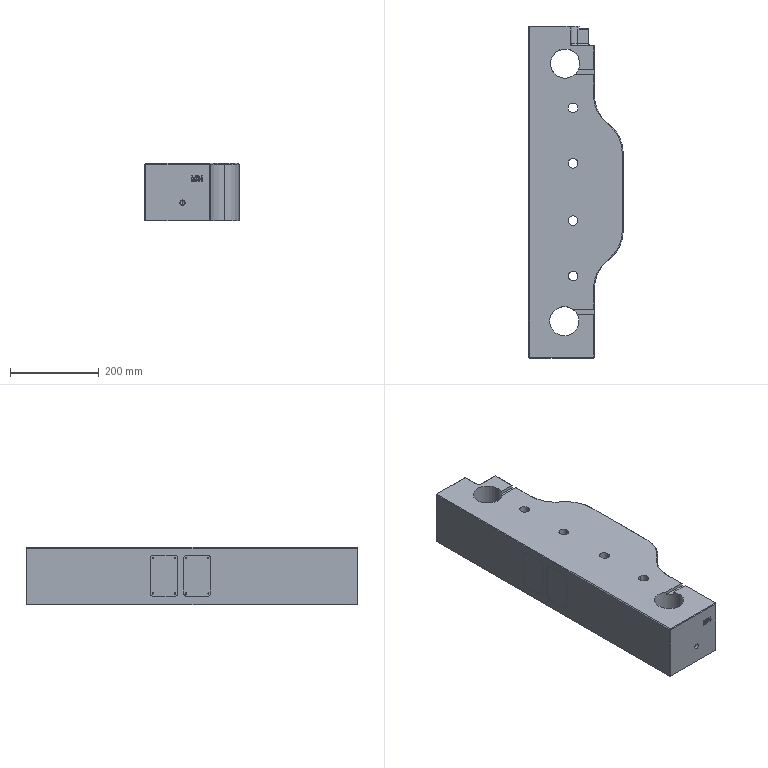Part | Creo | 1 solid | 380 faces | box 213 x 750 x 130 mm | volume 15709329 mm3 | plane 167 | other 90 | cylinder 78 | cone 44 | torus 1 | commonest cylinder face diameters 2.5 x16 14 x8 22 x8 6 x7 12 x6 16 x4